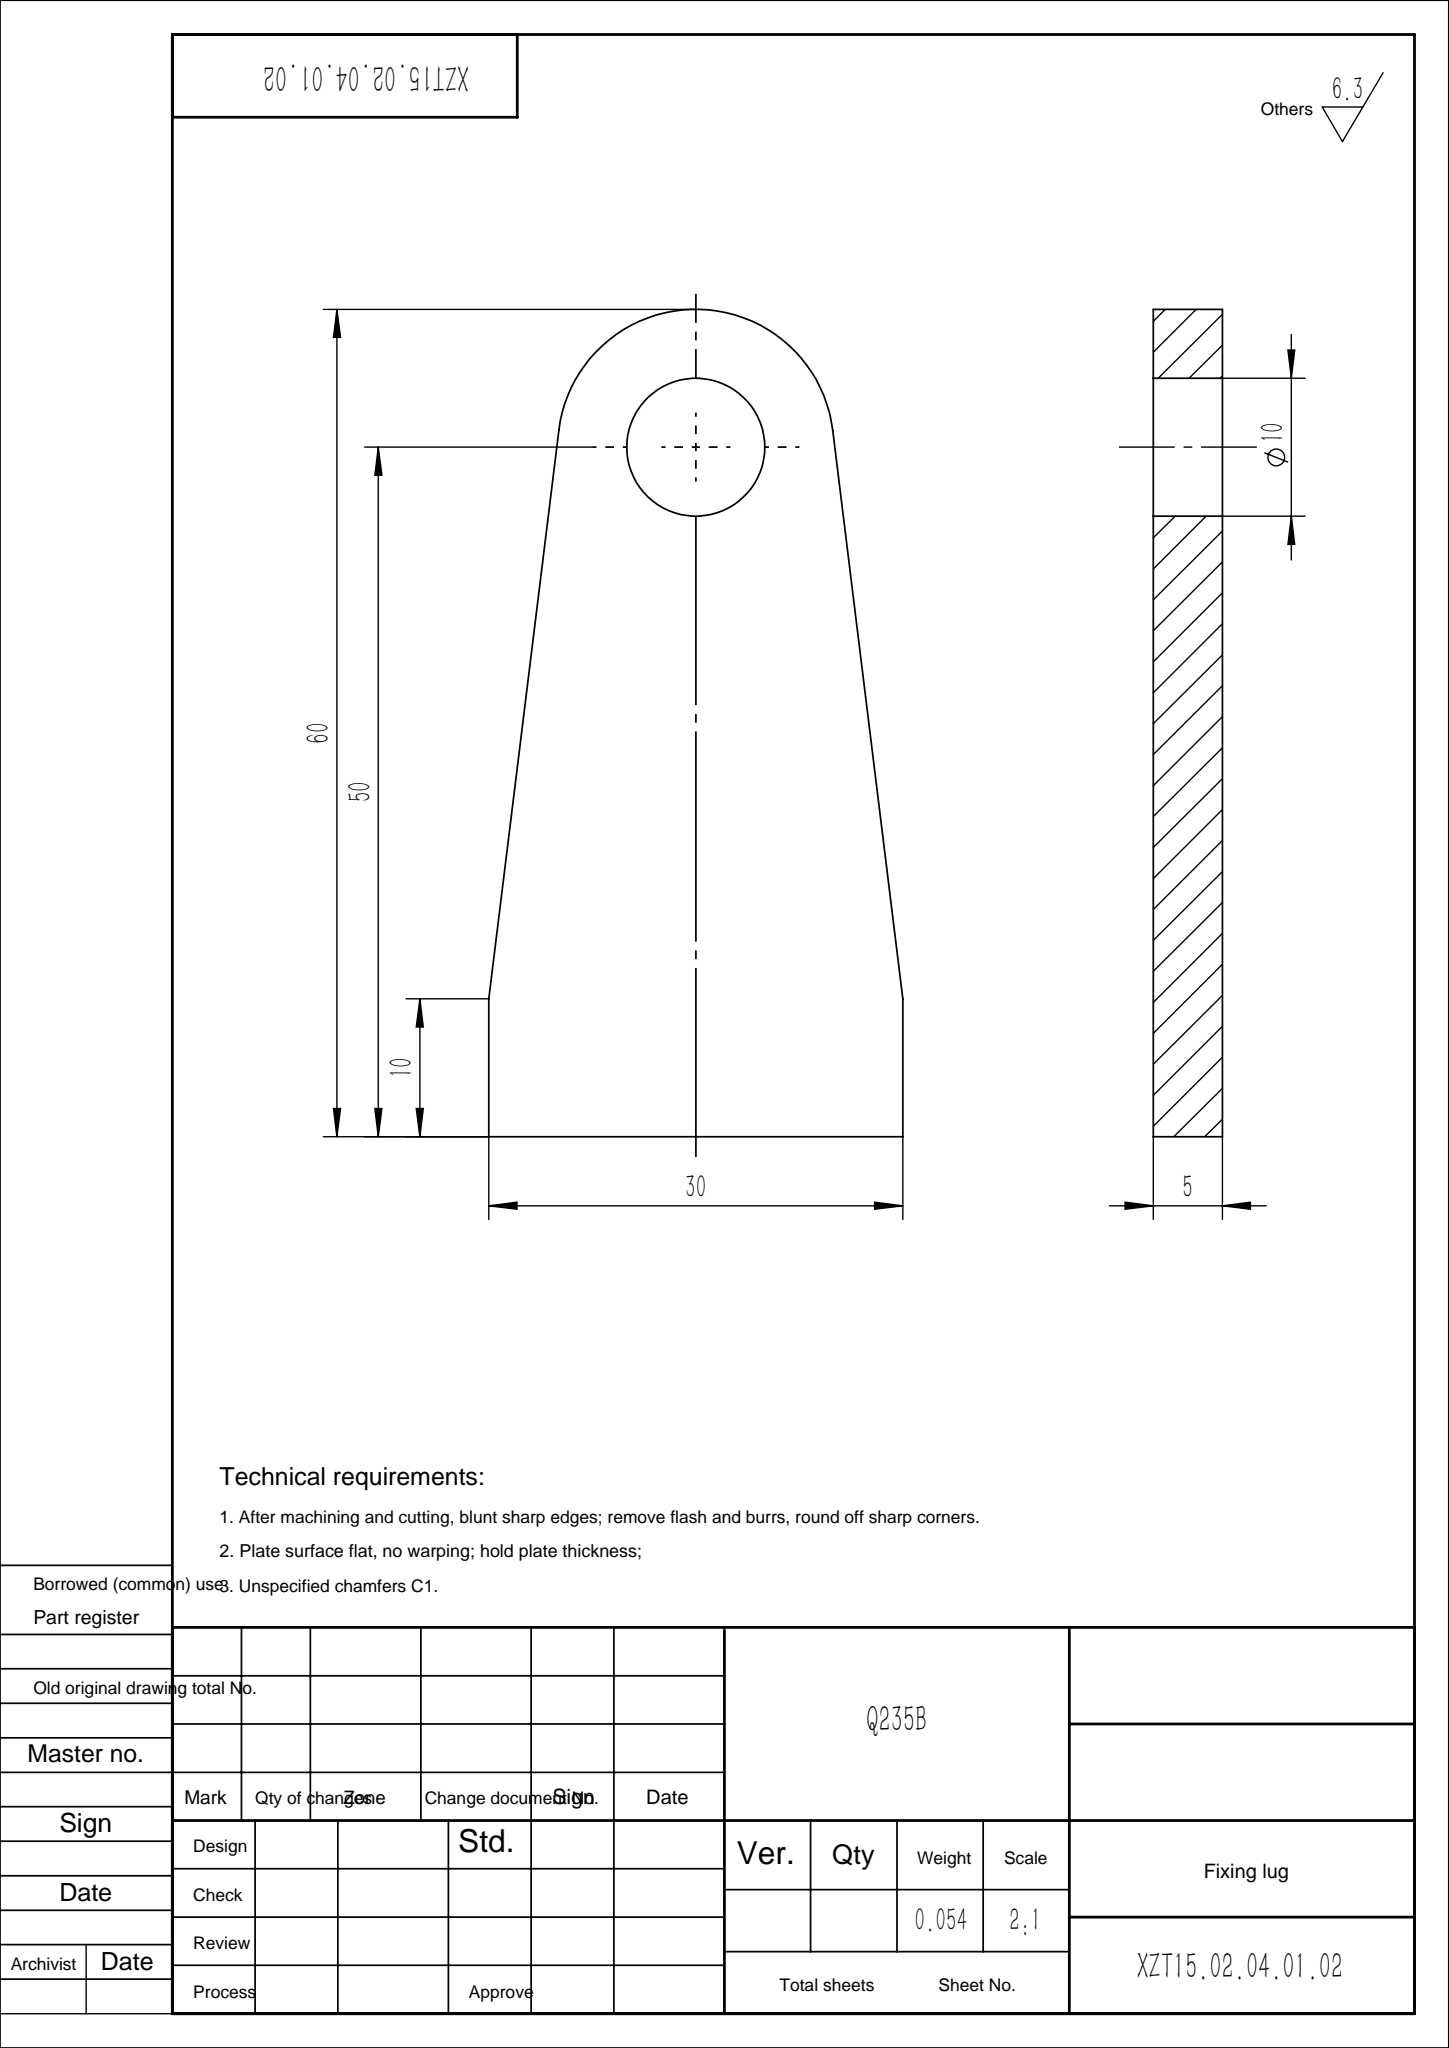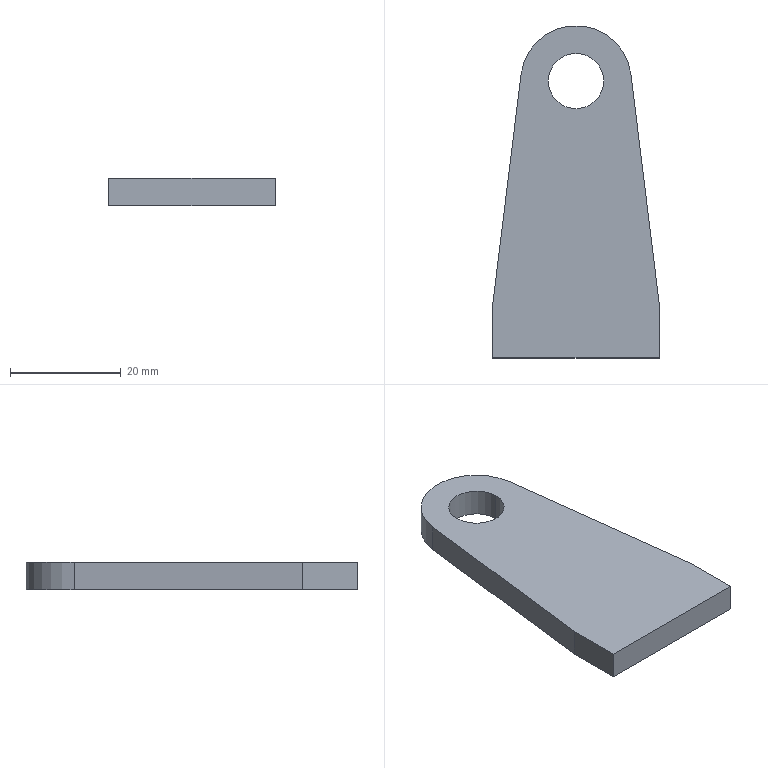Part | SolidWorks | features Extrusion 1, ICE 1 | 1 solid | 10 faces | box 30 x 60 x 5 mm | volume 6908 mm3 | plane 7 | cylinder 3 | commonest cylinder face diameters 10 x2 20 x1
STEP:
#1=CARTESIAN_POINT('',(-5.,40.,2.5));
#2=VERTEX_POINT('',#1);
#3=CARTESIAN_POINT('',(5.,40.,2.5));
#4=VERTEX_POINT('',#3);
#5=CARTESIAN_POINT('',(0.,40.,2.5));
#6=DIRECTION('',(0.,0.,1.));
#7=DIRECTION('',(1.,0.,0.));
#8=AXIS2_PLACEMENT_3D('',#5,#6,#7);
#9=CIRCLE('',#8,5.);
#10=EDGE_CURVE('',#2,#4,#9,.T.);
#11=ORIENTED_EDGE('',*,*,#10,.T.);
#12=CARTESIAN_POINT('',(5.,40.,-2.5));
#13=VERTEX_POINT('',#12);
#14=CARTESIAN_POINT('',(5.,40.,2.5));
#15=DIRECTION('',(0.,0.,-1.));
#16=VECTOR('',#15,1000.);
#17=LINE('',#14,#16);
#18=EDGE_CURVE('',#4,#13,#17,.T.);
#19=ORIENTED_EDGE('',*,*,#18,.T.);
#20=CARTESIAN_POINT('',(-5.,40.,-2.5));
#21=VERTEX_POINT('',#20);
#22=CARTESIAN_POINT('',(0.,40.,-2.5));
#23=DIRECTION('',(0.,0.,1.));
#24=DIRECTION('',(1.,0.,0.));
#25=AXIS2_PLACEMENT_3D('',#22,#23,#24);
#26=CIRCLE('',#25,5.);
#27=EDGE_CURVE('',#21,#13,#26,.T.);
#28=ORIENTED_EDGE('',*,*,#27,.F.);
#29=CARTESIAN_POINT('',(-5.,40.,2.5));
#30=DIRECTION('',(0.,0.,-1.));
#31=VECTOR('',#30,1000.);
#32=LINE('',#29,#31);
#33=EDGE_CURVE('',#2,#21,#32,.T.);
#34=ORIENTED_EDGE('',*,*,#33,.F.);
#35=EDGE_LOOP('',(#11,#19,#28,#34));
#36=FACE_OUTER_BOUND('',#35,.T.);
#37=CARTESIAN_POINT('',(0.,40.,2.5));
#38=DIRECTION('',(0.,0.,-1.));
#39=DIRECTION('',(-1.,0.,0.));
#40=AXIS2_PLACEMENT_3D('',#37,#38,#39);
#41=CYLINDRICAL_SURFACE('',#40,5.);
#42=ADVANCED_FACE('',(#36),#41,.F.);
#43=CARTESIAN_POINT('',(-9.925,41.222,2.5));
#44=VERTEX_POINT('',#43);
#45=CARTESIAN_POINT('',(-15.,0.,2.5));
#46=VERTEX_POINT('',#45);
#47=CARTESIAN_POINT('',(-15.,0.,2.5));
#48=DIRECTION('',(-0.1222,-0.9925,0.));
#49=VECTOR('',#48,1000.);
#50=LINE('',#47,#49);
#51=EDGE_CURVE('',#44,#46,#50,.T.);
#52=ORIENTED_EDGE('',*,*,#51,.T.);
#53=CARTESIAN_POINT('',(-15.,-10.,2.5));
#54=VERTEX_POINT('',#53);
#55=CARTESIAN_POINT('',(-15.,0.,2.5));
#56=DIRECTION('',(0.,-1.,0.));
#57=VECTOR('',#56,1000.);
#58=LINE('',#55,#57);
#59=EDGE_CURVE('',#46,#54,#58,.T.);
#60=ORIENTED_EDGE('',*,*,#59,.T.);
#61=CARTESIAN_POINT('',(15.,-10.,2.5));
#62=VERTEX_POINT('',#61);
#63=CARTESIAN_POINT('',(-15.,-10.,2.5));
#64=DIRECTION('',(1.,0.,0.));
#65=VECTOR('',#64,1000.);
#66=LINE('',#63,#65);
#67=EDGE_CURVE('',#54,#62,#66,.T.);
#68=ORIENTED_EDGE('',*,*,#67,.T.);
#69=CARTESIAN_POINT('',(15.,0.,2.5));
#70=VERTEX_POINT('',#69);
#71=CARTESIAN_POINT('',(15.,0.,2.5));
#72=DIRECTION('',(0.,1.,0.));
#73=VECTOR('',#72,1000.);
#74=LINE('',#71,#73);
#75=EDGE_CURVE('',#62,#70,#74,.T.);
#76=ORIENTED_EDGE('',*,*,#75,.T.);
#77=CARTESIAN_POINT('',(9.925,41.222,2.5));
#78=VERTEX_POINT('',#77);
#79=CARTESIAN_POINT('',(15.,0.,2.5));
#80=DIRECTION('',(-0.1222,0.9925,0.));
#81=VECTOR('',#80,1000.);
#82=LINE('',#79,#81);
#83=EDGE_CURVE('',#70,#78,#82,.T.);
#84=ORIENTED_EDGE('',*,*,#83,.T.);
#85=CARTESIAN_POINT('',(0.,40.,2.5));
#86=DIRECTION('',(0.,0.,1.));
#87=DIRECTION('',(-1.,0.,0.));
#88=AXIS2_PLACEMENT_3D('',#85,#86,#87);
#89=CIRCLE('',#88,10.);
#90=EDGE_CURVE('',#78,#44,#89,.T.);
#91=ORIENTED_EDGE('',*,*,#90,.T.);
#92=EDGE_LOOP('',(#52,#60,#68,#76,#84,#91));
#93=FACE_OUTER_BOUND('',#92,.T.);
#94=ORIENTED_EDGE('',*,*,#10,.F.);
#95=CARTESIAN_POINT('',(0.,40.,2.5));
#96=DIRECTION('',(0.,0.,1.));
#97=DIRECTION('',(1.,0.,0.));
#98=AXIS2_PLACEMENT_3D('',#95,#96,#97);
#99=CIRCLE('',#98,5.);
#100=EDGE_CURVE('',#4,#2,#99,.T.);
#101=ORIENTED_EDGE('',*,*,#100,.F.);
#102=EDGE_LOOP('',(#94,#101));
#103=FACE_BOUND('',#102,.T.);
#104=CARTESIAN_POINT('',(0.,40.,2.5));
#105=DIRECTION('',(0.,0.,-1.));
#106=DIRECTION('',(-1.,0.,0.));
#107=AXIS2_PLACEMENT_3D('',#104,#105,#106);
#108=PLANE('',#107);
#109=ADVANCED_FACE('',(#93,#103),#108,.F.);
#110=CARTESIAN_POINT('',(-9.925,41.222,-2.5));
#111=VERTEX_POINT('',#110);
#112=CARTESIAN_POINT('',(-15.,0.,-2.5));
#113=VERTEX_POINT('',#112);
#114=CARTESIAN_POINT('',(-15.,0.,-2.5));
#115=DIRECTION('',(-0.1222,-0.9925,0.));
#116=VECTOR('',#115,1000.);
#117=LINE('',#114,#116);
#118=EDGE_CURVE('',#111,#113,#117,.T.);
#119=ORIENTED_EDGE('',*,*,#118,.F.);
#120=CARTESIAN_POINT('',(9.925,41.222,-2.5));
#121=VERTEX_POINT('',#120);
#122=CARTESIAN_POINT('',(0.,40.,-2.5));
#123=DIRECTION('',(0.,0.,1.));
#124=DIRECTION('',(-1.,0.,0.));
#125=AXIS2_PLACEMENT_3D('',#122,#123,#124);
#126=CIRCLE('',#125,10.);
#127=EDGE_CURVE('',#121,#111,#126,.T.);
#128=ORIENTED_EDGE('',*,*,#127,.F.);
#129=CARTESIAN_POINT('',(15.,0.,-2.5));
#130=VERTEX_POINT('',#129);
#131=CARTESIAN_POINT('',(15.,0.,-2.5));
#132=DIRECTION('',(-0.1222,0.9925,0.));
#133=VECTOR('',#132,1000.);
#134=LINE('',#131,#133);
#135=EDGE_CURVE('',#130,#121,#134,.T.);
#136=ORIENTED_EDGE('',*,*,#135,.F.);
#137=CARTESIAN_POINT('',(15.,-10.,-2.5));
#138=VERTEX_POINT('',#137);
#139=CARTESIAN_POINT('',(15.,0.,-2.5));
#140=DIRECTION('',(0.,1.,0.));
#141=VECTOR('',#140,1000.);
#142=LINE('',#139,#141);
#143=EDGE_CURVE('',#138,#130,#142,.T.);
#144=ORIENTED_EDGE('',*,*,#143,.F.);
#145=CARTESIAN_POINT('',(-15.,-10.,-2.5));
#146=VERTEX_POINT('',#145);
#147=CARTESIAN_POINT('',(-15.,-10.,-2.5));
#148=DIRECTION('',(1.,0.,0.));
#149=VECTOR('',#148,1000.);
#150=LINE('',#147,#149);
#151=EDGE_CURVE('',#146,#138,#150,.T.);
#152=ORIENTED_EDGE('',*,*,#151,.F.);
#153=CARTESIAN_POINT('',(-15.,0.,-2.5));
#154=DIRECTION('',(0.,-1.,0.));
#155=VECTOR('',#154,1000.);
#156=LINE('',#153,#155);
#157=EDGE_CURVE('',#113,#146,#156,.T.);
#158=ORIENTED_EDGE('',*,*,#157,.F.);
#159=EDGE_LOOP('',(#119,#128,#136,#144,#152,#158));
#160=FACE_OUTER_BOUND('',#159,.T.);
#161=ORIENTED_EDGE('',*,*,#27,.T.);
#162=CARTESIAN_POINT('',(0.,40.,-2.5));
#163=DIRECTION('',(0.,0.,1.));
#164=DIRECTION('',(1.,0.,0.));
#165=AXIS2_PLACEMENT_3D('',#162,#163,#164);
#166=CIRCLE('',#165,5.);
#167=EDGE_CURVE('',#13,#21,#166,.T.);
#168=ORIENTED_EDGE('',*,*,#167,.T.);
#169=EDGE_LOOP('',(#161,#168));
#170=FACE_BOUND('',#169,.T.);
#171=CARTESIAN_POINT('',(0.,40.,-2.5));
#172=DIRECTION('',(0.,0.,-1.));
#173=DIRECTION('',(-1.,0.,0.));
#174=AXIS2_PLACEMENT_3D('',#171,#172,#173);
#175=PLANE('',#174);
#176=ADVANCED_FACE('',(#160,#170),#175,.T.);
#177=ORIENTED_EDGE('',*,*,#118,.T.);
#178=CARTESIAN_POINT('',(-15.,0.,2.5));
#179=DIRECTION('',(0.,0.,-1.));
#180=VECTOR('',#179,1000.);
#181=LINE('',#178,#180);
#182=EDGE_CURVE('',#46,#113,#181,.T.);
#183=ORIENTED_EDGE('',*,*,#182,.F.);
#184=ORIENTED_EDGE('',*,*,#51,.F.);
#185=CARTESIAN_POINT('',(-9.925,41.222,2.5));
#186=DIRECTION('',(0.,0.,-1.));
#187=VECTOR('',#186,1000.);
#188=LINE('',#185,#187);
#189=EDGE_CURVE('',#44,#111,#188,.T.);
#190=ORIENTED_EDGE('',*,*,#189,.T.);
#191=EDGE_LOOP('',(#177,#183,#184,#190));
#192=FACE_OUTER_BOUND('',#191,.T.);
#193=CARTESIAN_POINT('',(-15.,0.,2.5));
#194=DIRECTION('',(0.9925,-0.1222,0.));
#195=DIRECTION('',(0.1222,0.9925,0.));
#196=AXIS2_PLACEMENT_3D('',#193,#194,#195);
#197=PLANE('',#196);
#198=ADVANCED_FACE('',(#192),#197,.F.);
#199=ORIENTED_EDGE('',*,*,#135,.T.);
#200=CARTESIAN_POINT('',(9.925,41.222,2.5));
#201=DIRECTION('',(0.,0.,-1.));
#202=VECTOR('',#201,1000.);
#203=LINE('',#200,#202);
#204=EDGE_CURVE('',#78,#121,#203,.T.);
#205=ORIENTED_EDGE('',*,*,#204,.F.);
#206=ORIENTED_EDGE('',*,*,#83,.F.);
#207=CARTESIAN_POINT('',(15.,0.,2.5));
#208=DIRECTION('',(0.,0.,-1.));
#209=VECTOR('',#208,1000.);
#210=LINE('',#207,#209);
#211=EDGE_CURVE('',#70,#130,#210,.T.);
#212=ORIENTED_EDGE('',*,*,#211,.T.);
#213=EDGE_LOOP('',(#199,#205,#206,#212));
#214=FACE_OUTER_BOUND('',#213,.T.);
#215=CARTESIAN_POINT('',(15.,0.,2.5));
#216=DIRECTION('',(-0.9925,-0.1222,0.));
#217=DIRECTION('',(0.1222,-0.9925,0.));
#218=AXIS2_PLACEMENT_3D('',#215,#216,#217);
#219=PLANE('',#218);
#220=ADVANCED_FACE('',(#214),#219,.F.);
#221=ORIENTED_EDGE('',*,*,#127,.T.);
#222=ORIENTED_EDGE('',*,*,#189,.F.);
#223=ORIENTED_EDGE('',*,*,#90,.F.);
#224=ORIENTED_EDGE('',*,*,#204,.T.);
#225=EDGE_LOOP('',(#221,#222,#223,#224));
#226=FACE_OUTER_BOUND('',#225,.T.);
#227=CARTESIAN_POINT('',(0.,40.,2.5));
#228=DIRECTION('',(0.,0.,-1.));
#229=DIRECTION('',(-1.,0.,0.));
#230=AXIS2_PLACEMENT_3D('',#227,#228,#229);
#231=CYLINDRICAL_SURFACE('',#230,10.);
#232=ADVANCED_FACE('',(#226),#231,.T.);
#233=ORIENTED_EDGE('',*,*,#18,.F.);
#234=ORIENTED_EDGE('',*,*,#100,.T.);
#235=ORIENTED_EDGE('',*,*,#33,.T.);
#236=ORIENTED_EDGE('',*,*,#167,.F.);
#237=EDGE_LOOP('',(#233,#234,#235,#236));
#238=FACE_OUTER_BOUND('',#237,.T.);
#239=CARTESIAN_POINT('',(0.,40.,2.5));
#240=DIRECTION('',(0.,0.,-1.));
#241=DIRECTION('',(-1.,0.,0.));
#242=AXIS2_PLACEMENT_3D('',#239,#240,#241);
#243=CYLINDRICAL_SURFACE('',#242,5.);
#244=ADVANCED_FACE('',(#238),#243,.F.);
#245=ORIENTED_EDGE('',*,*,#59,.F.);
#246=ORIENTED_EDGE('',*,*,#182,.T.);
#247=ORIENTED_EDGE('',*,*,#157,.T.);
#248=CARTESIAN_POINT('',(-15.,-10.,-2.5));
#249=DIRECTION('',(0.,0.,1.));
#250=VECTOR('',#249,1000.);
#251=LINE('',#248,#250);
#252=EDGE_CURVE('',#146,#54,#251,.T.);
#253=ORIENTED_EDGE('',*,*,#252,.T.);
#254=EDGE_LOOP('',(#245,#246,#247,#253));
#255=FACE_OUTER_BOUND('',#254,.T.);
#256=CARTESIAN_POINT('',(-15.,0.,-2.5));
#257=DIRECTION('',(-1.,0.,0.));
#258=DIRECTION('',(0.,-1.,0.));
#259=AXIS2_PLACEMENT_3D('',#256,#257,#258);
#260=PLANE('',#259);
#261=ADVANCED_FACE('',(#255),#260,.T.);
#262=ORIENTED_EDGE('',*,*,#75,.F.);
#263=CARTESIAN_POINT('',(15.,-10.,-2.5));
#264=DIRECTION('',(0.,0.,1.));
#265=VECTOR('',#264,1000.);
#266=LINE('',#263,#265);
#267=EDGE_CURVE('',#138,#62,#266,.T.);
#268=ORIENTED_EDGE('',*,*,#267,.F.);
#269=ORIENTED_EDGE('',*,*,#143,.T.);
#270=ORIENTED_EDGE('',*,*,#211,.F.);
#271=EDGE_LOOP('',(#262,#268,#269,#270));
#272=FACE_OUTER_BOUND('',#271,.T.);
#273=CARTESIAN_POINT('',(15.,0.,-2.5));
#274=DIRECTION('',(1.,0.,0.));
#275=DIRECTION('',(0.,1.,0.));
#276=AXIS2_PLACEMENT_3D('',#273,#274,#275);
#277=PLANE('',#276);
#278=ADVANCED_FACE('',(#272),#277,.T.);
#279=ORIENTED_EDGE('',*,*,#67,.F.);
#280=ORIENTED_EDGE('',*,*,#252,.F.);
#281=ORIENTED_EDGE('',*,*,#151,.T.);
#282=ORIENTED_EDGE('',*,*,#267,.T.);
#283=EDGE_LOOP('',(#279,#280,#281,#282));
#284=FACE_OUTER_BOUND('',#283,.T.);
#285=CARTESIAN_POINT('',(-15.,-10.,-2.5));
#286=DIRECTION('',(0.,-1.,0.));
#287=DIRECTION('',(0.,0.,-1.));
#288=AXIS2_PLACEMENT_3D('',#285,#286,#287);
#289=PLANE('',#288);
#290=ADVANCED_FACE('',(#284),#289,.T.);
#291=CLOSED_SHELL('',(#42,#109,#176,#198,#220,#232,#244,#261,#278,#290));
#292=MANIFOLD_SOLID_BREP('',#291);
#293=CARTESIAN_POINT('',(0.,0.,0.));
#294=DIRECTION('',(0.,0.,1.));
#295=DIRECTION('',(1.,0.,0.));
#296=AXIS2_PLACEMENT_3D('',#293,#294,#295);
#297=(LENGTH_UNIT()NAMED_UNIT(*)SI_UNIT(.MILLI.,.METRE.));
#298=UNCERTAINTY_MEASURE_WITH_UNIT(LENGTH_MEASURE(0.00001),#297,'','');
#299=(NAMED_UNIT(*)PLANE_ANGLE_UNIT()SI_UNIT($,.RADIAN.));
#300=(NAMED_UNIT(*)SI_UNIT($,.STERADIAN.)SOLID_ANGLE_UNIT());
#301=(GEOMETRIC_REPRESENTATION_CONTEXT(3)GLOBAL_UNCERTAINTY_ASSIGNED_CONTEXT((#298))GLOBAL_UNIT_ASSIGNED_CONTEXT((#297,#299,#300))REPRESENTATION_CONTEXT('',''));
#302=ADVANCED_BREP_SHAPE_REPRESENTATION('',(#292,#296),#301);